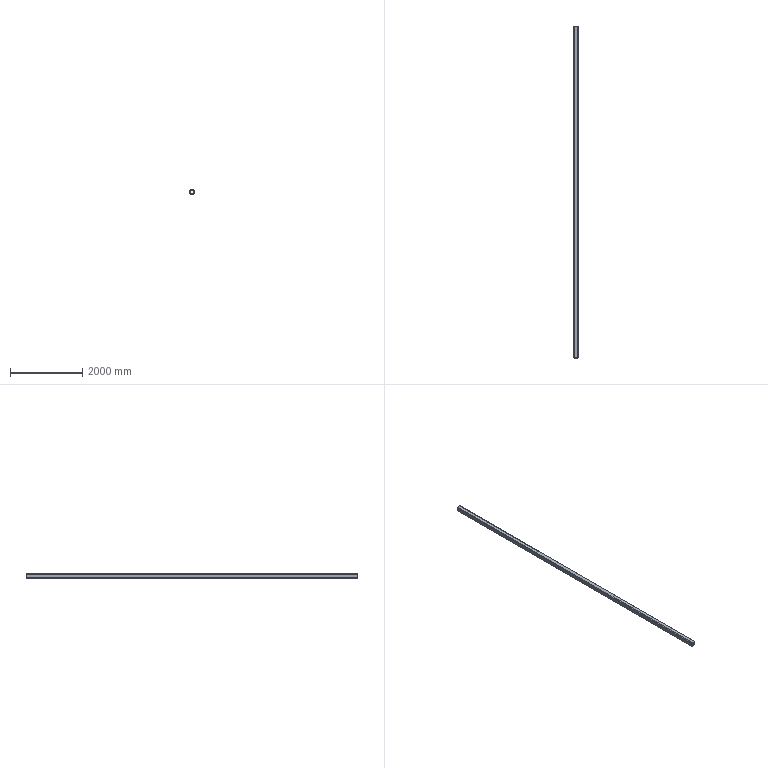Part | SolidWorks | features WeldMemberFeat 1, WeldmentFeature 1 | 1 solid | 18 faces | box 120 x 9220 x 120 mm | volume 38826807 mm3 | plane 10 | cylinder 8 | commonest cylinder face diameters 12 x4 32 x4
STEP:
#1=CARTESIAN_POINT('',(-60.,0.,44.));
#2=VERTEX_POINT('',#1);
#3=CARTESIAN_POINT('',(-44.,0.,60.));
#4=VERTEX_POINT('',#3);
#5=CARTESIAN_POINT('',(-44.,0.,44.));
#6=DIRECTION('',(0.,1.,0.));
#7=DIRECTION('',(0.,0.,1.));
#8=AXIS2_PLACEMENT_3D('',#5,#6,#7);
#9=CIRCLE('',#8,16.);
#10=EDGE_CURVE('',#2,#4,#9,.T.);
#11=ORIENTED_EDGE('',*,*,#10,.T.);
#12=CARTESIAN_POINT('',(-44.,9220.,60.));
#13=VERTEX_POINT('',#12);
#14=CARTESIAN_POINT('',(-44.,9220.,60.));
#15=DIRECTION('',(0.,-1.,0.));
#16=VECTOR('',#15,1000.);
#17=LINE('',#14,#16);
#18=EDGE_CURVE('',#13,#4,#17,.T.);
#19=ORIENTED_EDGE('',*,*,#18,.F.);
#20=CARTESIAN_POINT('',(-60.,9220.,44.));
#21=VERTEX_POINT('',#20);
#22=CARTESIAN_POINT('',(-44.,9220.,44.));
#23=DIRECTION('',(0.,1.,0.));
#24=DIRECTION('',(0.,0.,1.));
#25=AXIS2_PLACEMENT_3D('',#22,#23,#24);
#26=CIRCLE('',#25,16.);
#27=EDGE_CURVE('',#21,#13,#26,.T.);
#28=ORIENTED_EDGE('',*,*,#27,.F.);
#29=CARTESIAN_POINT('',(-60.,9220.,44.));
#30=DIRECTION('',(0.,-1.,0.));
#31=VECTOR('',#30,1000.);
#32=LINE('',#29,#31);
#33=EDGE_CURVE('',#21,#2,#32,.T.);
#34=ORIENTED_EDGE('',*,*,#33,.T.);
#35=EDGE_LOOP('',(#11,#19,#28,#34));
#36=FACE_OUTER_BOUND('',#35,.T.);
#37=CARTESIAN_POINT('',(-44.,9220.,44.));
#38=DIRECTION('',(0.,-1.,0.));
#39=DIRECTION('',(0.,0.,-1.));
#40=AXIS2_PLACEMENT_3D('',#37,#38,#39);
#41=CYLINDRICAL_SURFACE('',#40,16.);
#42=ADVANCED_FACE('',(#36),#41,.T.);
#43=CARTESIAN_POINT('',(44.,0.,60.));
#44=VERTEX_POINT('',#43);
#45=CARTESIAN_POINT('',(-44.,0.,60.));
#46=DIRECTION('',(1.,0.,0.));
#47=VECTOR('',#46,1000.);
#48=LINE('',#45,#47);
#49=EDGE_CURVE('',#4,#44,#48,.T.);
#50=ORIENTED_EDGE('',*,*,#49,.T.);
#51=CARTESIAN_POINT('',(44.,9220.,60.));
#52=VERTEX_POINT('',#51);
#53=CARTESIAN_POINT('',(44.,9220.,60.));
#54=DIRECTION('',(0.,-1.,0.));
#55=VECTOR('',#54,1000.);
#56=LINE('',#53,#55);
#57=EDGE_CURVE('',#52,#44,#56,.T.);
#58=ORIENTED_EDGE('',*,*,#57,.F.);
#59=CARTESIAN_POINT('',(-44.,9220.,60.));
#60=DIRECTION('',(1.,0.,0.));
#61=VECTOR('',#60,1000.);
#62=LINE('',#59,#61);
#63=EDGE_CURVE('',#13,#52,#62,.T.);
#64=ORIENTED_EDGE('',*,*,#63,.F.);
#65=ORIENTED_EDGE('',*,*,#18,.T.);
#66=EDGE_LOOP('',(#50,#58,#64,#65));
#67=FACE_OUTER_BOUND('',#66,.T.);
#68=CARTESIAN_POINT('',(-44.,9220.,60.));
#69=DIRECTION('',(0.,0.,-1.));
#70=DIRECTION('',(-1.,0.,0.));
#71=AXIS2_PLACEMENT_3D('',#68,#69,#70);
#72=PLANE('',#71);
#73=ADVANCED_FACE('',(#67),#72,.F.);
#74=CARTESIAN_POINT('',(60.,0.,44.));
#75=VERTEX_POINT('',#74);
#76=CARTESIAN_POINT('',(44.,0.,44.));
#77=DIRECTION('',(0.,1.,0.));
#78=DIRECTION('',(0.,0.,1.));
#79=AXIS2_PLACEMENT_3D('',#76,#77,#78);
#80=CIRCLE('',#79,16.);
#81=EDGE_CURVE('',#44,#75,#80,.T.);
#82=ORIENTED_EDGE('',*,*,#81,.T.);
#83=CARTESIAN_POINT('',(60.,9220.,44.));
#84=VERTEX_POINT('',#83);
#85=CARTESIAN_POINT('',(60.,9220.,44.));
#86=DIRECTION('',(0.,-1.,0.));
#87=VECTOR('',#86,1000.);
#88=LINE('',#85,#87);
#89=EDGE_CURVE('',#84,#75,#88,.T.);
#90=ORIENTED_EDGE('',*,*,#89,.F.);
#91=CARTESIAN_POINT('',(44.,9220.,44.));
#92=DIRECTION('',(0.,1.,0.));
#93=DIRECTION('',(0.,0.,1.));
#94=AXIS2_PLACEMENT_3D('',#91,#92,#93);
#95=CIRCLE('',#94,16.);
#96=EDGE_CURVE('',#52,#84,#95,.T.);
#97=ORIENTED_EDGE('',*,*,#96,.F.);
#98=ORIENTED_EDGE('',*,*,#57,.T.);
#99=EDGE_LOOP('',(#82,#90,#97,#98));
#100=FACE_OUTER_BOUND('',#99,.T.);
#101=CARTESIAN_POINT('',(44.,9220.,44.));
#102=DIRECTION('',(0.,-1.,0.));
#103=DIRECTION('',(0.,0.,-1.));
#104=AXIS2_PLACEMENT_3D('',#101,#102,#103);
#105=CYLINDRICAL_SURFACE('',#104,16.);
#106=ADVANCED_FACE('',(#100),#105,.T.);
#107=CARTESIAN_POINT('',(60.,0.,-44.));
#108=VERTEX_POINT('',#107);
#109=CARTESIAN_POINT('',(60.,0.,-44.));
#110=DIRECTION('',(0.,0.,-1.));
#111=VECTOR('',#110,1000.);
#112=LINE('',#109,#111);
#113=EDGE_CURVE('',#75,#108,#112,.T.);
#114=ORIENTED_EDGE('',*,*,#113,.T.);
#115=CARTESIAN_POINT('',(60.,9220.,-44.));
#116=VERTEX_POINT('',#115);
#117=CARTESIAN_POINT('',(60.,9220.,-44.));
#118=DIRECTION('',(0.,-1.,0.));
#119=VECTOR('',#118,1000.);
#120=LINE('',#117,#119);
#121=EDGE_CURVE('',#116,#108,#120,.T.);
#122=ORIENTED_EDGE('',*,*,#121,.F.);
#123=CARTESIAN_POINT('',(60.,9220.,-44.));
#124=DIRECTION('',(0.,0.,-1.));
#125=VECTOR('',#124,1000.);
#126=LINE('',#123,#125);
#127=EDGE_CURVE('',#84,#116,#126,.T.);
#128=ORIENTED_EDGE('',*,*,#127,.F.);
#129=ORIENTED_EDGE('',*,*,#89,.T.);
#130=EDGE_LOOP('',(#114,#122,#128,#129));
#131=FACE_OUTER_BOUND('',#130,.T.);
#132=CARTESIAN_POINT('',(60.,9220.,-44.));
#133=DIRECTION('',(-1.,0.,0.));
#134=DIRECTION('',(0.,0.,1.));
#135=AXIS2_PLACEMENT_3D('',#132,#133,#134);
#136=PLANE('',#135);
#137=ADVANCED_FACE('',(#131),#136,.F.);
#138=CARTESIAN_POINT('',(44.,0.,-60.));
#139=VERTEX_POINT('',#138);
#140=CARTESIAN_POINT('',(44.,0.,-44.));
#141=DIRECTION('',(0.,1.,0.));
#142=DIRECTION('',(0.,0.,1.));
#143=AXIS2_PLACEMENT_3D('',#140,#141,#142);
#144=CIRCLE('',#143,16.);
#145=EDGE_CURVE('',#108,#139,#144,.T.);
#146=ORIENTED_EDGE('',*,*,#145,.T.);
#147=CARTESIAN_POINT('',(44.,9220.,-60.));
#148=VERTEX_POINT('',#147);
#149=CARTESIAN_POINT('',(44.,9220.,-60.));
#150=DIRECTION('',(0.,-1.,0.));
#151=VECTOR('',#150,1000.);
#152=LINE('',#149,#151);
#153=EDGE_CURVE('',#148,#139,#152,.T.);
#154=ORIENTED_EDGE('',*,*,#153,.F.);
#155=CARTESIAN_POINT('',(44.,9220.,-44.));
#156=DIRECTION('',(0.,1.,0.));
#157=DIRECTION('',(0.,0.,1.));
#158=AXIS2_PLACEMENT_3D('',#155,#156,#157);
#159=CIRCLE('',#158,16.);
#160=EDGE_CURVE('',#116,#148,#159,.T.);
#161=ORIENTED_EDGE('',*,*,#160,.F.);
#162=ORIENTED_EDGE('',*,*,#121,.T.);
#163=EDGE_LOOP('',(#146,#154,#161,#162));
#164=FACE_OUTER_BOUND('',#163,.T.);
#165=CARTESIAN_POINT('',(44.,9220.,-44.));
#166=DIRECTION('',(0.,-1.,0.));
#167=DIRECTION('',(0.,0.,-1.));
#168=AXIS2_PLACEMENT_3D('',#165,#166,#167);
#169=CYLINDRICAL_SURFACE('',#168,16.);
#170=ADVANCED_FACE('',(#164),#169,.T.);
#171=CARTESIAN_POINT('',(-44.,0.,-60.));
#172=VERTEX_POINT('',#171);
#173=CARTESIAN_POINT('',(44.,0.,-60.));
#174=DIRECTION('',(-1.,0.,0.));
#175=VECTOR('',#174,1000.);
#176=LINE('',#173,#175);
#177=EDGE_CURVE('',#139,#172,#176,.T.);
#178=ORIENTED_EDGE('',*,*,#177,.T.);
#179=CARTESIAN_POINT('',(-44.,9220.,-60.));
#180=VERTEX_POINT('',#179);
#181=CARTESIAN_POINT('',(-44.,9220.,-60.));
#182=DIRECTION('',(0.,-1.,0.));
#183=VECTOR('',#182,1000.);
#184=LINE('',#181,#183);
#185=EDGE_CURVE('',#180,#172,#184,.T.);
#186=ORIENTED_EDGE('',*,*,#185,.F.);
#187=CARTESIAN_POINT('',(44.,9220.,-60.));
#188=DIRECTION('',(-1.,0.,0.));
#189=VECTOR('',#188,1000.);
#190=LINE('',#187,#189);
#191=EDGE_CURVE('',#148,#180,#190,.T.);
#192=ORIENTED_EDGE('',*,*,#191,.F.);
#193=ORIENTED_EDGE('',*,*,#153,.T.);
#194=EDGE_LOOP('',(#178,#186,#192,#193));
#195=FACE_OUTER_BOUND('',#194,.T.);
#196=CARTESIAN_POINT('',(44.,9220.,-60.));
#197=DIRECTION('',(0.,0.,1.));
#198=DIRECTION('',(1.,0.,0.));
#199=AXIS2_PLACEMENT_3D('',#196,#197,#198);
#200=PLANE('',#199);
#201=ADVANCED_FACE('',(#195),#200,.F.);
#202=CARTESIAN_POINT('',(-60.,0.,-44.));
#203=VERTEX_POINT('',#202);
#204=CARTESIAN_POINT('',(-44.,0.,-44.));
#205=DIRECTION('',(0.,1.,0.));
#206=DIRECTION('',(0.,0.,1.));
#207=AXIS2_PLACEMENT_3D('',#204,#205,#206);
#208=CIRCLE('',#207,16.);
#209=EDGE_CURVE('',#172,#203,#208,.T.);
#210=ORIENTED_EDGE('',*,*,#209,.T.);
#211=CARTESIAN_POINT('',(-60.,9220.,-44.));
#212=VERTEX_POINT('',#211);
#213=CARTESIAN_POINT('',(-60.,9220.,-44.));
#214=DIRECTION('',(0.,-1.,0.));
#215=VECTOR('',#214,1000.);
#216=LINE('',#213,#215);
#217=EDGE_CURVE('',#212,#203,#216,.T.);
#218=ORIENTED_EDGE('',*,*,#217,.F.);
#219=CARTESIAN_POINT('',(-44.,9220.,-44.));
#220=DIRECTION('',(0.,1.,0.));
#221=DIRECTION('',(0.,0.,1.));
#222=AXIS2_PLACEMENT_3D('',#219,#220,#221);
#223=CIRCLE('',#222,16.);
#224=EDGE_CURVE('',#180,#212,#223,.T.);
#225=ORIENTED_EDGE('',*,*,#224,.F.);
#226=ORIENTED_EDGE('',*,*,#185,.T.);
#227=EDGE_LOOP('',(#210,#218,#225,#226));
#228=FACE_OUTER_BOUND('',#227,.T.);
#229=CARTESIAN_POINT('',(-44.,9220.,-44.));
#230=DIRECTION('',(0.,-1.,0.));
#231=DIRECTION('',(0.,0.,-1.));
#232=AXIS2_PLACEMENT_3D('',#229,#230,#231);
#233=CYLINDRICAL_SURFACE('',#232,16.);
#234=ADVANCED_FACE('',(#228),#233,.T.);
#235=CARTESIAN_POINT('',(44.,0.,50.));
#236=VERTEX_POINT('',#235);
#237=CARTESIAN_POINT('',(50.,0.,44.));
#238=VERTEX_POINT('',#237);
#239=CARTESIAN_POINT('',(44.,0.,44.));
#240=DIRECTION('',(0.,1.,0.));
#241=DIRECTION('',(0.,0.,1.));
#242=AXIS2_PLACEMENT_3D('',#239,#240,#241);
#243=CIRCLE('',#242,6.);
#244=EDGE_CURVE('',#236,#238,#243,.T.);
#245=ORIENTED_EDGE('',*,*,#244,.F.);
#246=CARTESIAN_POINT('',(44.,9220.,50.));
#247=VERTEX_POINT('',#246);
#248=CARTESIAN_POINT('',(44.,9220.,50.));
#249=DIRECTION('',(0.,-1.,0.));
#250=VECTOR('',#249,1000.);
#251=LINE('',#248,#250);
#252=EDGE_CURVE('',#247,#236,#251,.T.);
#253=ORIENTED_EDGE('',*,*,#252,.F.);
#254=CARTESIAN_POINT('',(50.,9220.,44.));
#255=VERTEX_POINT('',#254);
#256=CARTESIAN_POINT('',(44.,9220.,44.));
#257=DIRECTION('',(0.,1.,0.));
#258=DIRECTION('',(0.,0.,1.));
#259=AXIS2_PLACEMENT_3D('',#256,#257,#258);
#260=CIRCLE('',#259,6.);
#261=EDGE_CURVE('',#247,#255,#260,.T.);
#262=ORIENTED_EDGE('',*,*,#261,.T.);
#263=CARTESIAN_POINT('',(50.,9220.,44.));
#264=DIRECTION('',(0.,-1.,0.));
#265=VECTOR('',#264,1000.);
#266=LINE('',#263,#265);
#267=EDGE_CURVE('',#255,#238,#266,.T.);
#268=ORIENTED_EDGE('',*,*,#267,.T.);
#269=EDGE_LOOP('',(#245,#253,#262,#268));
#270=FACE_OUTER_BOUND('',#269,.T.);
#271=CARTESIAN_POINT('',(44.,9220.,44.));
#272=DIRECTION('',(0.,-1.,0.));
#273=DIRECTION('',(0.,0.,-1.));
#274=AXIS2_PLACEMENT_3D('',#271,#272,#273);
#275=CYLINDRICAL_SURFACE('',#274,6.);
#276=ADVANCED_FACE('',(#270),#275,.F.);
#277=CARTESIAN_POINT('',(-44.,0.,50.));
#278=VERTEX_POINT('',#277);
#279=CARTESIAN_POINT('',(-44.,0.,50.));
#280=DIRECTION('',(1.,0.,0.));
#281=VECTOR('',#280,1000.);
#282=LINE('',#279,#281);
#283=EDGE_CURVE('',#278,#236,#282,.T.);
#284=ORIENTED_EDGE('',*,*,#283,.F.);
#285=CARTESIAN_POINT('',(-44.,9220.,50.));
#286=VERTEX_POINT('',#285);
#287=CARTESIAN_POINT('',(-44.,9220.,50.));
#288=DIRECTION('',(0.,-1.,0.));
#289=VECTOR('',#288,1000.);
#290=LINE('',#287,#289);
#291=EDGE_CURVE('',#286,#278,#290,.T.);
#292=ORIENTED_EDGE('',*,*,#291,.F.);
#293=CARTESIAN_POINT('',(-44.,9220.,50.));
#294=DIRECTION('',(1.,0.,0.));
#295=VECTOR('',#294,1000.);
#296=LINE('',#293,#295);
#297=EDGE_CURVE('',#286,#247,#296,.T.);
#298=ORIENTED_EDGE('',*,*,#297,.T.);
#299=ORIENTED_EDGE('',*,*,#252,.T.);
#300=EDGE_LOOP('',(#284,#292,#298,#299));
#301=FACE_OUTER_BOUND('',#300,.T.);
#302=CARTESIAN_POINT('',(-44.,9220.,50.));
#303=DIRECTION('',(0.,0.,-1.));
#304=DIRECTION('',(-1.,0.,0.));
#305=AXIS2_PLACEMENT_3D('',#302,#303,#304);
#306=PLANE('',#305);
#307=ADVANCED_FACE('',(#301),#306,.T.);
#308=CARTESIAN_POINT('',(-50.,0.,44.));
#309=VERTEX_POINT('',#308);
#310=CARTESIAN_POINT('',(-44.,0.,44.));
#311=DIRECTION('',(0.,1.,0.));
#312=DIRECTION('',(0.,0.,1.));
#313=AXIS2_PLACEMENT_3D('',#310,#311,#312);
#314=CIRCLE('',#313,6.);
#315=EDGE_CURVE('',#309,#278,#314,.T.);
#316=ORIENTED_EDGE('',*,*,#315,.F.);
#317=CARTESIAN_POINT('',(-50.,9220.,44.));
#318=VERTEX_POINT('',#317);
#319=CARTESIAN_POINT('',(-50.,9220.,44.));
#320=DIRECTION('',(0.,-1.,0.));
#321=VECTOR('',#320,1000.);
#322=LINE('',#319,#321);
#323=EDGE_CURVE('',#318,#309,#322,.T.);
#324=ORIENTED_EDGE('',*,*,#323,.F.);
#325=CARTESIAN_POINT('',(-44.,9220.,44.));
#326=DIRECTION('',(0.,1.,0.));
#327=DIRECTION('',(0.,0.,1.));
#328=AXIS2_PLACEMENT_3D('',#325,#326,#327);
#329=CIRCLE('',#328,6.);
#330=EDGE_CURVE('',#318,#286,#329,.T.);
#331=ORIENTED_EDGE('',*,*,#330,.T.);
#332=ORIENTED_EDGE('',*,*,#291,.T.);
#333=EDGE_LOOP('',(#316,#324,#331,#332));
#334=FACE_OUTER_BOUND('',#333,.T.);
#335=CARTESIAN_POINT('',(-44.,9220.,44.));
#336=DIRECTION('',(0.,-1.,0.));
#337=DIRECTION('',(0.,0.,-1.));
#338=AXIS2_PLACEMENT_3D('',#335,#336,#337);
#339=CYLINDRICAL_SURFACE('',#338,6.);
#340=ADVANCED_FACE('',(#334),#339,.F.);
#341=CARTESIAN_POINT('',(-50.,0.,-44.));
#342=VERTEX_POINT('',#341);
#343=CARTESIAN_POINT('',(-50.,0.,44.));
#344=DIRECTION('',(0.,0.,1.));
#345=VECTOR('',#344,1000.);
#346=LINE('',#343,#345);
#347=EDGE_CURVE('',#342,#309,#346,.T.);
#348=ORIENTED_EDGE('',*,*,#347,.F.);
#349=CARTESIAN_POINT('',(-50.,9220.,-44.));
#350=VERTEX_POINT('',#349);
#351=CARTESIAN_POINT('',(-50.,9220.,-44.));
#352=DIRECTION('',(0.,-1.,0.));
#353=VECTOR('',#352,1000.);
#354=LINE('',#351,#353);
#355=EDGE_CURVE('',#350,#342,#354,.T.);
#356=ORIENTED_EDGE('',*,*,#355,.F.);
#357=CARTESIAN_POINT('',(-50.,9220.,44.));
#358=DIRECTION('',(0.,0.,1.));
#359=VECTOR('',#358,1000.);
#360=LINE('',#357,#359);
#361=EDGE_CURVE('',#350,#318,#360,.T.);
#362=ORIENTED_EDGE('',*,*,#361,.T.);
#363=ORIENTED_EDGE('',*,*,#323,.T.);
#364=EDGE_LOOP('',(#348,#356,#362,#363));
#365=FACE_OUTER_BOUND('',#364,.T.);
#366=CARTESIAN_POINT('',(-50.,9220.,44.));
#367=DIRECTION('',(1.,0.,0.));
#368=DIRECTION('',(0.,0.,-1.));
#369=AXIS2_PLACEMENT_3D('',#366,#367,#368);
#370=PLANE('',#369);
#371=ADVANCED_FACE('',(#365),#370,.T.);
#372=CARTESIAN_POINT('',(-44.,0.,-50.));
#373=VERTEX_POINT('',#372);
#374=CARTESIAN_POINT('',(-44.,0.,-44.));
#375=DIRECTION('',(0.,1.,0.));
#376=DIRECTION('',(0.,0.,1.));
#377=AXIS2_PLACEMENT_3D('',#374,#375,#376);
#378=CIRCLE('',#377,6.);
#379=EDGE_CURVE('',#373,#342,#378,.T.);
#380=ORIENTED_EDGE('',*,*,#379,.F.);
#381=CARTESIAN_POINT('',(-44.,9220.,-50.));
#382=VERTEX_POINT('',#381);
#383=CARTESIAN_POINT('',(-44.,9220.,-50.));
#384=DIRECTION('',(0.,-1.,0.));
#385=VECTOR('',#384,1000.);
#386=LINE('',#383,#385);
#387=EDGE_CURVE('',#382,#373,#386,.T.);
#388=ORIENTED_EDGE('',*,*,#387,.F.);
#389=CARTESIAN_POINT('',(-44.,9220.,-44.));
#390=DIRECTION('',(0.,1.,0.));
#391=DIRECTION('',(0.,0.,1.));
#392=AXIS2_PLACEMENT_3D('',#389,#390,#391);
#393=CIRCLE('',#392,6.);
#394=EDGE_CURVE('',#382,#350,#393,.T.);
#395=ORIENTED_EDGE('',*,*,#394,.T.);
#396=ORIENTED_EDGE('',*,*,#355,.T.);
#397=EDGE_LOOP('',(#380,#388,#395,#396));
#398=FACE_OUTER_BOUND('',#397,.T.);
#399=CARTESIAN_POINT('',(-44.,9220.,-44.));
#400=DIRECTION('',(0.,-1.,0.));
#401=DIRECTION('',(0.,0.,-1.));
#402=AXIS2_PLACEMENT_3D('',#399,#400,#401);
#403=CYLINDRICAL_SURFACE('',#402,6.);
#404=ADVANCED_FACE('',(#398),#403,.F.);
#405=CARTESIAN_POINT('',(44.,0.,-50.));
#406=VERTEX_POINT('',#405);
#407=CARTESIAN_POINT('',(44.,0.,-50.));
#408=DIRECTION('',(-1.,0.,0.));
#409=VECTOR('',#408,1000.);
#410=LINE('',#407,#409);
#411=EDGE_CURVE('',#406,#373,#410,.T.);
#412=ORIENTED_EDGE('',*,*,#411,.F.);
#413=CARTESIAN_POINT('',(44.,9220.,-50.));
#414=VERTEX_POINT('',#413);
#415=CARTESIAN_POINT('',(44.,9220.,-50.));
#416=DIRECTION('',(0.,-1.,0.));
#417=VECTOR('',#416,1000.);
#418=LINE('',#415,#417);
#419=EDGE_CURVE('',#414,#406,#418,.T.);
#420=ORIENTED_EDGE('',*,*,#419,.F.);
#421=CARTESIAN_POINT('',(44.,9220.,-50.));
#422=DIRECTION('',(-1.,0.,0.));
#423=VECTOR('',#422,1000.);
#424=LINE('',#421,#423);
#425=EDGE_CURVE('',#414,#382,#424,.T.);
#426=ORIENTED_EDGE('',*,*,#425,.T.);
#427=ORIENTED_EDGE('',*,*,#387,.T.);
#428=EDGE_LOOP('',(#412,#420,#426,#427));
#429=FACE_OUTER_BOUND('',#428,.T.);
#430=CARTESIAN_POINT('',(44.,9220.,-50.));
#431=DIRECTION('',(0.,0.,1.));
#432=DIRECTION('',(1.,0.,0.));
#433=AXIS2_PLACEMENT_3D('',#430,#431,#432);
#434=PLANE('',#433);
#435=ADVANCED_FACE('',(#429),#434,.T.);
#436=CARTESIAN_POINT('',(50.,0.,-44.));
#437=VERTEX_POINT('',#436);
#438=CARTESIAN_POINT('',(44.,0.,-44.));
#439=DIRECTION('',(0.,1.,0.));
#440=DIRECTION('',(0.,0.,1.));
#441=AXIS2_PLACEMENT_3D('',#438,#439,#440);
#442=CIRCLE('',#441,6.);
#443=EDGE_CURVE('',#437,#406,#442,.T.);
#444=ORIENTED_EDGE('',*,*,#443,.F.);
#445=CARTESIAN_POINT('',(50.,9220.,-44.));
#446=VERTEX_POINT('',#445);
#447=CARTESIAN_POINT('',(50.,9220.,-44.));
#448=DIRECTION('',(0.,-1.,0.));
#449=VECTOR('',#448,1000.);
#450=LINE('',#447,#449);
#451=EDGE_CURVE('',#446,#437,#450,.T.);
#452=ORIENTED_EDGE('',*,*,#451,.F.);
#453=CARTESIAN_POINT('',(44.,9220.,-44.));
#454=DIRECTION('',(0.,1.,0.));
#455=DIRECTION('',(0.,0.,1.));
#456=AXIS2_PLACEMENT_3D('',#453,#454,#455);
#457=CIRCLE('',#456,6.);
#458=EDGE_CURVE('',#446,#414,#457,.T.);
#459=ORIENTED_EDGE('',*,*,#458,.T.);
#460=ORIENTED_EDGE('',*,*,#419,.T.);
#461=EDGE_LOOP('',(#444,#452,#459,#460));
#462=FACE_OUTER_BOUND('',#461,.T.);
#463=CARTESIAN_POINT('',(44.,9220.,-44.));
#464=DIRECTION('',(0.,-1.,0.));
#465=DIRECTION('',(0.,0.,-1.));
#466=AXIS2_PLACEMENT_3D('',#463,#464,#465);
#467=CYLINDRICAL_SURFACE('',#466,6.);
#468=ADVANCED_FACE('',(#462),#467,.F.);
#469=CARTESIAN_POINT('',(50.,0.,-44.));
#470=DIRECTION('',(0.,0.,-1.));
#471=VECTOR('',#470,1000.);
#472=LINE('',#469,#471);
#473=EDGE_CURVE('',#238,#437,#472,.T.);
#474=ORIENTED_EDGE('',*,*,#473,.F.);
#475=ORIENTED_EDGE('',*,*,#267,.F.);
#476=CARTESIAN_POINT('',(50.,9220.,-44.));
#477=DIRECTION('',(0.,0.,-1.));
#478=VECTOR('',#477,1000.);
#479=LINE('',#476,#478);
#480=EDGE_CURVE('',#255,#446,#479,.T.);
#481=ORIENTED_EDGE('',*,*,#480,.T.);
#482=ORIENTED_EDGE('',*,*,#451,.T.);
#483=EDGE_LOOP('',(#474,#475,#481,#482));
#484=FACE_OUTER_BOUND('',#483,.T.);
#485=CARTESIAN_POINT('',(50.,9220.,-44.));
#486=DIRECTION('',(-1.,0.,0.));
#487=DIRECTION('',(0.,0.,1.));
#488=AXIS2_PLACEMENT_3D('',#485,#486,#487);
#489=PLANE('',#488);
#490=ADVANCED_FACE('',(#484),#489,.T.);
#491=CARTESIAN_POINT('',(-60.,0.,44.));
#492=DIRECTION('',(0.,0.,1.));
#493=VECTOR('',#492,1000.);
#494=LINE('',#491,#493);
#495=EDGE_CURVE('',#203,#2,#494,.T.);
#496=ORIENTED_EDGE('',*,*,#495,.T.);
#497=ORIENTED_EDGE('',*,*,#33,.F.);
#498=CARTESIAN_POINT('',(-60.,9220.,44.));
#499=DIRECTION('',(0.,0.,1.));
#500=VECTOR('',#499,1000.);
#501=LINE('',#498,#500);
#502=EDGE_CURVE('',#212,#21,#501,.T.);
#503=ORIENTED_EDGE('',*,*,#502,.F.);
#504=ORIENTED_EDGE('',*,*,#217,.T.);
#505=EDGE_LOOP('',(#496,#497,#503,#504));
#506=FACE_OUTER_BOUND('',#505,.T.);
#507=CARTESIAN_POINT('',(-60.,9220.,44.));
#508=DIRECTION('',(1.,0.,0.));
#509=DIRECTION('',(0.,0.,-1.));
#510=AXIS2_PLACEMENT_3D('',#507,#508,#509);
#511=PLANE('',#510);
#512=ADVANCED_FACE('',(#506),#511,.F.);
#513=ORIENTED_EDGE('',*,*,#261,.F.);
#514=ORIENTED_EDGE('',*,*,#297,.F.);
#515=ORIENTED_EDGE('',*,*,#330,.F.);
#516=ORIENTED_EDGE('',*,*,#361,.F.);
#517=ORIENTED_EDGE('',*,*,#394,.F.);
#518=ORIENTED_EDGE('',*,*,#425,.F.);
#519=ORIENTED_EDGE('',*,*,#458,.F.);
#520=ORIENTED_EDGE('',*,*,#480,.F.);
#521=EDGE_LOOP('',(#513,#514,#515,#516,#517,#518,#519,#520));
#522=FACE_BOUND('',#521,.T.);
#523=ORIENTED_EDGE('',*,*,#27,.T.);
#524=ORIENTED_EDGE('',*,*,#63,.T.);
#525=ORIENTED_EDGE('',*,*,#96,.T.);
#526=ORIENTED_EDGE('',*,*,#127,.T.);
#527=ORIENTED_EDGE('',*,*,#160,.T.);
#528=ORIENTED_EDGE('',*,*,#191,.T.);
#529=ORIENTED_EDGE('',*,*,#224,.T.);
#530=ORIENTED_EDGE('',*,*,#502,.T.);
#531=EDGE_LOOP('',(#523,#524,#525,#526,#527,#528,#529,#530));
#532=FACE_OUTER_BOUND('',#531,.T.);
#533=CARTESIAN_POINT('',(-44.,9220.,44.));
#534=DIRECTION('',(0.,1.,0.));
#535=DIRECTION('',(0.,0.,1.));
#536=AXIS2_PLACEMENT_3D('',#533,#534,#535);
#537=PLANE('',#536);
#538=ADVANCED_FACE('',(#522,#532),#537,.T.);
#539=ORIENTED_EDGE('',*,*,#244,.T.);
#540=ORIENTED_EDGE('',*,*,#473,.T.);
#541=ORIENTED_EDGE('',*,*,#443,.T.);
#542=ORIENTED_EDGE('',*,*,#411,.T.);
#543=ORIENTED_EDGE('',*,*,#379,.T.);
#544=ORIENTED_EDGE('',*,*,#347,.T.);
#545=ORIENTED_EDGE('',*,*,#315,.T.);
#546=ORIENTED_EDGE('',*,*,#283,.T.);
#547=EDGE_LOOP('',(#539,#540,#541,#542,#543,#544,#545,#546));
#548=FACE_BOUND('',#547,.T.);
#549=ORIENTED_EDGE('',*,*,#10,.F.);
#550=ORIENTED_EDGE('',*,*,#495,.F.);
#551=ORIENTED_EDGE('',*,*,#209,.F.);
#552=ORIENTED_EDGE('',*,*,#177,.F.);
#553=ORIENTED_EDGE('',*,*,#145,.F.);
#554=ORIENTED_EDGE('',*,*,#113,.F.);
#555=ORIENTED_EDGE('',*,*,#81,.F.);
#556=ORIENTED_EDGE('',*,*,#49,.F.);
#557=EDGE_LOOP('',(#549,#550,#551,#552,#553,#554,#555,#556));
#558=FACE_OUTER_BOUND('',#557,.T.);
#559=CARTESIAN_POINT('',(-44.,0.,44.));
#560=DIRECTION('',(0.,1.,0.));
#561=DIRECTION('',(0.,0.,1.));
#562=AXIS2_PLACEMENT_3D('',#559,#560,#561);
#563=PLANE('',#562);
#564=ADVANCED_FACE('',(#548,#558),#563,.F.);
#565=CLOSED_SHELL('',(#42,#73,#106,#137,#170,#201,#234,#276,#307,#340,#371,#404,#435,#468,#490,#512,#538,#564));
#566=MANIFOLD_SOLID_BREP('',#565);
#567=CARTESIAN_POINT('',(0.,0.,0.));
#568=DIRECTION('',(0.,0.,1.));
#569=DIRECTION('',(1.,0.,0.));
#570=AXIS2_PLACEMENT_3D('',#567,#568,#569);
#571=(LENGTH_UNIT()NAMED_UNIT(*)SI_UNIT(.MILLI.,.METRE.));
#572=UNCERTAINTY_MEASURE_WITH_UNIT(LENGTH_MEASURE(0.00001),#571,'','');
#573=(NAMED_UNIT(*)PLANE_ANGLE_UNIT()SI_UNIT($,.RADIAN.));
#574=(NAMED_UNIT(*)SI_UNIT($,.STERADIAN.)SOLID_ANGLE_UNIT());
#575=(GEOMETRIC_REPRESENTATION_CONTEXT(3)GLOBAL_UNCERTAINTY_ASSIGNED_CONTEXT((#572))GLOBAL_UNIT_ASSIGNED_CONTEXT((#571,#573,#574))REPRESENTATION_CONTEXT('',''));
#576=ADVANCED_BREP_SHAPE_REPRESENTATION('',(#566,#570),#575);